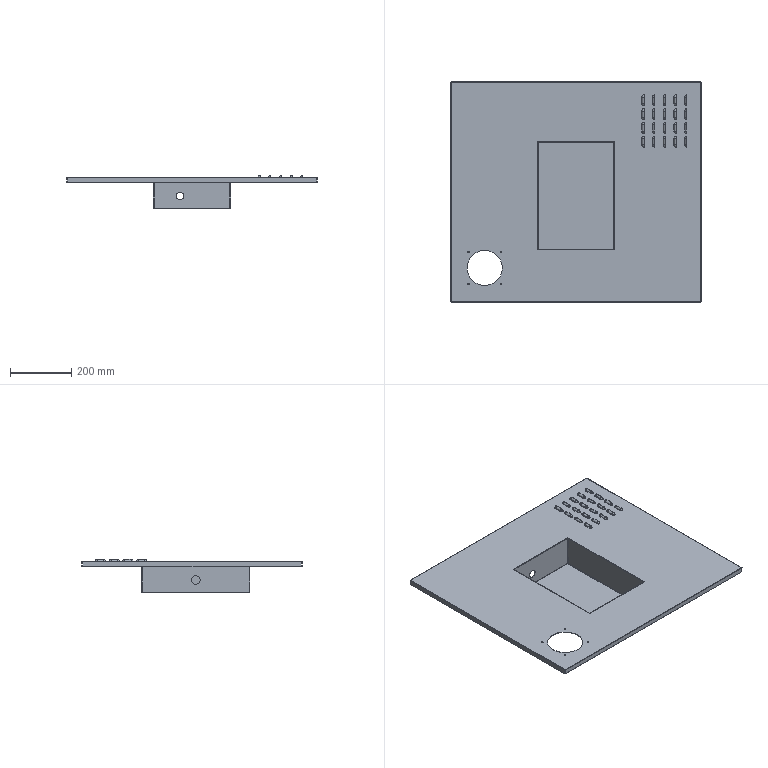Part | STEP file | Side cover plate | 1 solid | 378 faces | box 818 x 718 x 108.6 mm | volume 888983 mm3 | cylinder 114 | plane 88 | torus 80 | sphere 80 | spline 16 | commonest cylinder face diameters 1.6 x20 4 x20 12 x20 14.4 x20 0.4 x9 2.8 x9